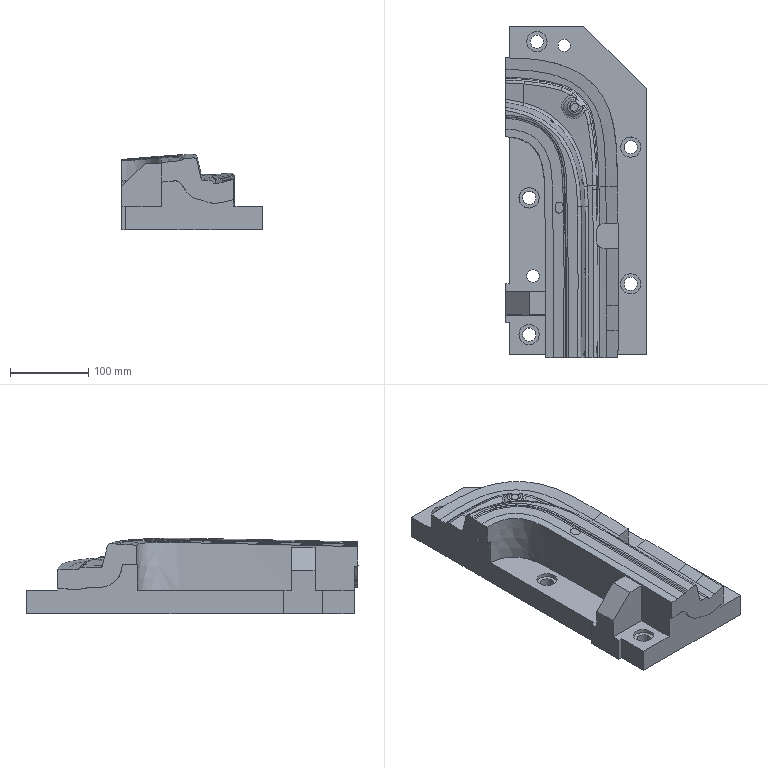Part | NX | features solid 2 | 1 solid | 112 faces | box 180 x 425 x 96.38 mm | volume 3881513 mm3 | spline 73 | plane 25 | cylinder 14 | commonest cylinder face diameters 17 x5 26 x5 16 x2 20 x2